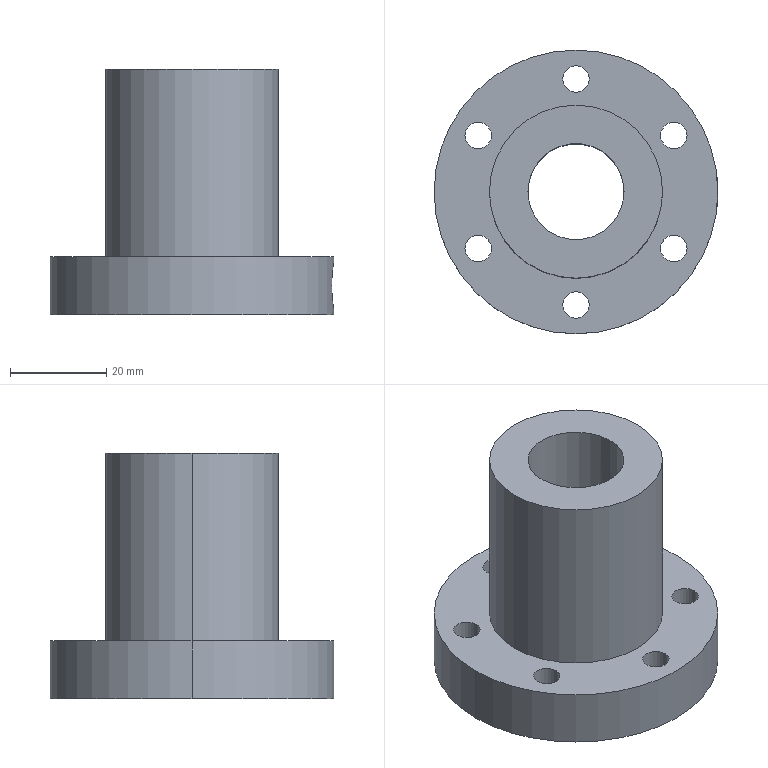Part | SolidWorks | features BaseBody 1 | 1 solid | 44 faces | box 59 x 59 x 51 mm | volume 51895 mm3 | cylinder 34 | plane 10 | commonest cylinder face diameters 5.5 x12 9.5 x12 8 x2 10 x2 20 x2 36 x2
STEP:
#1=CARTESIAN_POINT('',(-18.,0.,51.));
#2=VERTEX_POINT('',#1);
#3=CARTESIAN_POINT('',(18.,0.,51.));
#4=VERTEX_POINT('',#3);
#5=CARTESIAN_POINT('',(0.,0.,51.));
#6=DIRECTION('',(0.,0.,-1.));
#7=DIRECTION('',(-1.,0.,0.));
#8=AXIS2_PLACEMENT_3D('',#5,#6,#7);
#9=CIRCLE('',#8,18.);
#10=EDGE_CURVE('',#2,#4,#9,.T.);
#11=ORIENTED_EDGE('',*,*,#10,.T.);
#12=CARTESIAN_POINT('',(18.,0.,12.));
#13=VERTEX_POINT('',#12);
#14=CARTESIAN_POINT('',(18.,0.,-13.427));
#15=DIRECTION('',(0.,0.,-1.));
#16=VECTOR('',#15,1000.);
#17=LINE('',#14,#16);
#18=EDGE_CURVE('',#4,#13,#17,.T.);
#19=ORIENTED_EDGE('',*,*,#18,.T.);
#20=CARTESIAN_POINT('',(-18.,0.,12.));
#21=VERTEX_POINT('',#20);
#22=CARTESIAN_POINT('',(0.,0.,12.));
#23=DIRECTION('',(0.,0.,1.));
#24=DIRECTION('',(-1.,0.,0.));
#25=AXIS2_PLACEMENT_3D('',#22,#23,#24);
#26=CIRCLE('',#25,18.);
#27=EDGE_CURVE('',#13,#21,#26,.T.);
#28=ORIENTED_EDGE('',*,*,#27,.T.);
#29=CARTESIAN_POINT('',(-18.,0.,-13.427));
#30=DIRECTION('',(0.,0.,-1.));
#31=VECTOR('',#30,1000.);
#32=LINE('',#29,#31);
#33=EDGE_CURVE('',#2,#21,#32,.T.);
#34=ORIENTED_EDGE('',*,*,#33,.F.);
#35=EDGE_LOOP('',(#11,#19,#28,#34));
#36=FACE_OUTER_BOUND('',#35,.T.);
#37=CARTESIAN_POINT('',(0.,0.,-13.427));
#38=DIRECTION('',(0.,0.,-1.));
#39=DIRECTION('',(-1.,0.,0.));
#40=AXIS2_PLACEMENT_3D('',#37,#38,#39);
#41=CYLINDRICAL_SURFACE('',#40,18.);
#42=ADVANCED_FACE('',(#36),#41,.T.);
#43=CARTESIAN_POINT('',(-10.,0.,51.));
#44=VERTEX_POINT('',#43);
#45=CARTESIAN_POINT('',(10.,0.,51.));
#46=VERTEX_POINT('',#45);
#47=CARTESIAN_POINT('',(0.,0.,51.));
#48=DIRECTION('',(0.,0.,1.));
#49=DIRECTION('',(-1.,0.,0.));
#50=AXIS2_PLACEMENT_3D('',#47,#48,#49);
#51=CIRCLE('',#50,10.);
#52=EDGE_CURVE('',#44,#46,#51,.T.);
#53=ORIENTED_EDGE('',*,*,#52,.T.);
#54=CARTESIAN_POINT('',(10.,0.,10.));
#55=VERTEX_POINT('',#54);
#56=CARTESIAN_POINT('',(10.,0.,-13.427));
#57=DIRECTION('',(0.,0.,-1.));
#58=VECTOR('',#57,1000.);
#59=LINE('',#56,#58);
#60=EDGE_CURVE('',#46,#55,#59,.T.);
#61=ORIENTED_EDGE('',*,*,#60,.T.);
#62=CARTESIAN_POINT('',(10.,0.,2.));
#63=VERTEX_POINT('',#62);
#64=CARTESIAN_POINT('',(10.,0.,2.));
#65=CARTESIAN_POINT('',(10.,-0.2672,2.));
#66=CARTESIAN_POINT('',(9.989,-0.5294,2.026));
#67=CARTESIAN_POINT('',(9.949,-1.044,2.13));
#68=CARTESIAN_POINT('',(9.918,-1.3,2.208));
#69=CARTESIAN_POINT('',(9.843,-1.783,2.41));
#70=CARTESIAN_POINT('',(9.798,-2.012,2.533));
#71=CARTESIAN_POINT('',(9.699,-2.445,2.823));
#72=CARTESIAN_POINT('',(9.645,-2.647,2.99));
#73=CARTESIAN_POINT('',(9.538,-3.012,3.355));
#74=CARTESIAN_POINT('',(9.483,-3.177,3.555));
#75=CARTESIAN_POINT('',(9.381,-3.468,3.989));
#76=CARTESIAN_POINT('',(9.334,-3.59,4.218));
#77=CARTESIAN_POINT('',(9.254,-3.791,4.698));
#78=CARTESIAN_POINT('',(9.221,-3.869,4.952));
#79=CARTESIAN_POINT('',(9.177,-3.973,5.469));
#80=CARTESIAN_POINT('',(9.165,-4.,5.731));
#81=CARTESIAN_POINT('',(9.165,-4.,6.259));
#82=CARTESIAN_POINT('',(9.177,-3.974,6.527));
#83=CARTESIAN_POINT('',(9.221,-3.871,7.042));
#84=CARTESIAN_POINT('',(9.253,-3.794,7.293));
#85=CARTESIAN_POINT('',(9.333,-3.592,7.781));
#86=CARTESIAN_POINT('',(9.381,-3.468,8.009));
#87=CARTESIAN_POINT('',(9.482,-3.18,8.44));
#88=CARTESIAN_POINT('',(9.537,-3.013,8.643));
#89=CARTESIAN_POINT('',(9.645,-2.647,9.01));
#90=CARTESIAN_POINT('',(9.698,-2.448,9.174));
#91=CARTESIAN_POINT('',(9.797,-2.017,9.464));
#92=CARTESIAN_POINT('',(9.843,-1.784,9.59));
#93=CARTESIAN_POINT('',(9.918,-1.303,9.791));
#94=CARTESIAN_POINT('',(9.948,-1.054,9.868));
#95=CARTESIAN_POINT('',(9.989,-0.5328,9.973));
#96=CARTESIAN_POINT('',(10.,-0.2673,10.));
#97=CARTESIAN_POINT('',(10.,0.,10.));
#98=B_SPLINE_CURVE_WITH_KNOTS('',3,(#64,#65,#66,#67,#68,#69,#70,#71,#72,#73,#74,#75,#76,#77,#78,#79,#80,#81,#82,#83,#84,#85,#86,#87,#88,#89,#90,#91,#92,#93,#94,#95,#96,#97),.UNSPECIFIED.,.F.,.F.,(4,2,2,2,2,2,2,2,2,2,2,2,2,2,2,2,4),(0.,0.0007896,0.001579,0.002369,0.003158,0.003948,0.004738,0.005527,0.006317,0.007107,0.007896,0.008686,0.009475,0.01027,0.01105,0.01184,0.01263),.UNSPECIFIED.);
#99=EDGE_CURVE('',#63,#55,#98,.T.);
#100=ORIENTED_EDGE('',*,*,#99,.F.);
#101=CARTESIAN_POINT('',(10.,0.,0.));
#102=VERTEX_POINT('',#101);
#103=CARTESIAN_POINT('',(10.,0.,-13.427));
#104=DIRECTION('',(0.,0.,-1.));
#105=VECTOR('',#104,1000.);
#106=LINE('',#103,#105);
#107=EDGE_CURVE('',#63,#102,#106,.T.);
#108=ORIENTED_EDGE('',*,*,#107,.T.);
#109=CARTESIAN_POINT('',(-10.,0.,0.));
#110=VERTEX_POINT('',#109);
#111=CARTESIAN_POINT('',(0.,0.,0.));
#112=DIRECTION('',(0.,0.,1.));
#113=DIRECTION('',(-1.,0.,0.));
#114=AXIS2_PLACEMENT_3D('',#111,#112,#113);
#115=CIRCLE('',#114,10.);
#116=EDGE_CURVE('',#110,#102,#115,.T.);
#117=ORIENTED_EDGE('',*,*,#116,.F.);
#118=CARTESIAN_POINT('',(-10.,0.,-13.427));
#119=DIRECTION('',(0.,0.,-1.));
#120=VECTOR('',#119,1000.);
#121=LINE('',#118,#120);
#122=EDGE_CURVE('',#44,#110,#121,.T.);
#123=ORIENTED_EDGE('',*,*,#122,.F.);
#124=EDGE_LOOP('',(#53,#61,#100,#108,#117,#123));
#125=FACE_OUTER_BOUND('',#124,.T.);
#126=CARTESIAN_POINT('',(0.,0.,-13.427));
#127=DIRECTION('',(0.,0.,-1.));
#128=DIRECTION('',(-1.,0.,0.));
#129=AXIS2_PLACEMENT_3D('',#126,#127,#128);
#130=CYLINDRICAL_SURFACE('',#129,10.);
#131=ADVANCED_FACE('',(#125),#130,.F.);
#132=CARTESIAN_POINT('',(-29.5,0.,12.));
#133=VERTEX_POINT('',#132);
#134=CARTESIAN_POINT('',(29.5,0.,12.));
#135=VERTEX_POINT('',#134);
#136=CARTESIAN_POINT('',(0.,0.,12.));
#137=DIRECTION('',(0.,0.,-1.));
#138=DIRECTION('',(-1.,0.,0.));
#139=AXIS2_PLACEMENT_3D('',#136,#137,#138);
#140=CIRCLE('',#139,29.5);
#141=EDGE_CURVE('',#133,#135,#140,.T.);
#142=ORIENTED_EDGE('',*,*,#141,.T.);
#143=CARTESIAN_POINT('',(29.5,0.,11.));
#144=VERTEX_POINT('',#143);
#145=CARTESIAN_POINT('',(29.5,0.,-13.427));
#146=DIRECTION('',(0.,0.,-1.));
#147=VECTOR('',#146,1000.);
#148=LINE('',#145,#147);
#149=EDGE_CURVE('',#135,#144,#148,.T.);
#150=ORIENTED_EDGE('',*,*,#149,.T.);
#151=CARTESIAN_POINT('',(29.5,0.,1.));
#152=VERTEX_POINT('',#151);
#153=CARTESIAN_POINT('',(29.5,0.,11.));
#154=CARTESIAN_POINT('',(29.5,0.3309,11.));
#155=CARTESIAN_POINT('',(29.494,0.6562,10.967));
#156=CARTESIAN_POINT('',(29.479,1.136,10.872));
#157=CARTESIAN_POINT('',(29.472,1.295,10.832));
#158=CARTESIAN_POINT('',(29.457,1.609,10.737));
#159=CARTESIAN_POINT('',(29.448,1.765,10.681));
#160=CARTESIAN_POINT('',(29.418,2.219,10.493));
#161=CARTESIAN_POINT('',(29.395,2.506,10.339));
#162=CARTESIAN_POINT('',(29.343,3.049,9.976));
#163=CARTESIAN_POINT('',(29.315,3.306,9.766));
#164=CARTESIAN_POINT('',(29.26,3.766,9.305));
#165=CARTESIAN_POINT('',(29.232,3.973,9.054));
#166=CARTESIAN_POINT('',(29.18,4.338,8.508));
#167=CARTESIAN_POINT('',(29.156,4.493,8.218));
#168=CARTESIAN_POINT('',(29.117,4.743,7.617));
#169=CARTESIAN_POINT('',(29.1,4.839,7.301));
#170=CARTESIAN_POINT('',(29.079,4.968,6.655));
#171=CARTESIAN_POINT('',(29.073,5.,6.331));
#172=CARTESIAN_POINT('',(29.073,5.,5.677));
#173=CARTESIAN_POINT('',(29.079,4.968,5.345));
#174=CARTESIAN_POINT('',(29.1,4.84,4.704));
#175=CARTESIAN_POINT('',(29.116,4.746,4.392));
#176=CARTESIAN_POINT('',(29.146,4.558,3.937));
#177=CARTESIAN_POINT('',(29.157,4.487,3.787));
#178=CARTESIAN_POINT('',(29.18,4.332,3.498));
#179=CARTESIAN_POINT('',(29.193,4.248,3.358));
#180=CARTESIAN_POINT('',(29.231,3.977,2.953));
#181=CARTESIAN_POINT('',(29.259,3.77,2.699));
#182=CARTESIAN_POINT('',(29.315,3.305,2.234));
#183=CARTESIAN_POINT('',(29.343,3.053,2.027));
#184=CARTESIAN_POINT('',(29.394,2.513,1.665));
#185=CARTESIAN_POINT('',(29.418,2.22,1.508));
#186=CARTESIAN_POINT('',(29.457,1.616,1.257));
#187=CARTESIAN_POINT('',(29.473,1.304,1.162));
#188=CARTESIAN_POINT('',(29.494,0.6622,1.033));
#189=CARTESIAN_POINT('',(29.5,0.3309,1.));
#190=CARTESIAN_POINT('',(29.5,0.,1.));
#191=B_SPLINE_CURVE_WITH_KNOTS('',3,(#153,#154,#155,#156,#157,#158,#159,#160,#161,#162,#163,#164,#165,#166,#167,#168,#169,#170,#171,#172,#173,#174,#175,#176,#177,#178,#179,#180,#181,#182,#183,#184,#185,#186,#187,#188,#189,#190),.UNSPECIFIED.,.F.,.F.,(4,2,2,2,2,2,2,2,2,2,2,2,2,2,2,2,2,2,4),(0.,0.0009785,0.001468,0.001957,0.002936,0.003914,0.004893,0.005871,0.00685,0.007828,0.008807,0.009785,0.01027,0.01076,0.01174,0.01272,0.0137,0.01468,0.01566),.UNSPECIFIED.);
#192=EDGE_CURVE('',#144,#152,#191,.T.);
#193=ORIENTED_EDGE('',*,*,#192,.T.);
#194=CARTESIAN_POINT('',(29.5,0.,0.));
#195=VERTEX_POINT('',#194);
#196=CARTESIAN_POINT('',(29.5,0.,-13.427));
#197=DIRECTION('',(0.,0.,-1.));
#198=VECTOR('',#197,1000.);
#199=LINE('',#196,#198);
#200=EDGE_CURVE('',#152,#195,#199,.T.);
#201=ORIENTED_EDGE('',*,*,#200,.T.);
#202=CARTESIAN_POINT('',(-29.5,0.,0.));
#203=VERTEX_POINT('',#202);
#204=CARTESIAN_POINT('',(0.,0.,0.));
#205=DIRECTION('',(0.,0.,1.));
#206=DIRECTION('',(-1.,0.,0.));
#207=AXIS2_PLACEMENT_3D('',#204,#205,#206);
#208=CIRCLE('',#207,29.5);
#209=EDGE_CURVE('',#195,#203,#208,.T.);
#210=ORIENTED_EDGE('',*,*,#209,.T.);
#211=CARTESIAN_POINT('',(-29.5,0.,-13.427));
#212=DIRECTION('',(0.,0.,-1.));
#213=VECTOR('',#212,1000.);
#214=LINE('',#211,#213);
#215=EDGE_CURVE('',#133,#203,#214,.T.);
#216=ORIENTED_EDGE('',*,*,#215,.F.);
#217=EDGE_LOOP('',(#142,#150,#193,#201,#210,#216));
#218=FACE_OUTER_BOUND('',#217,.T.);
#219=CARTESIAN_POINT('',(0.,0.,-13.427));
#220=DIRECTION('',(0.,0.,-1.));
#221=DIRECTION('',(-1.,0.,0.));
#222=AXIS2_PLACEMENT_3D('',#219,#220,#221);
#223=CYLINDRICAL_SURFACE('',#222,29.5);
#224=ADVANCED_FACE('',(#218),#223,.T.);
#225=CARTESIAN_POINT('',(-2.75,23.5,5.5));
#226=VERTEX_POINT('',#225);
#227=CARTESIAN_POINT('',(2.75,23.5,5.5));
#228=VERTEX_POINT('',#227);
#229=CARTESIAN_POINT('',(0.,23.5,5.5));
#230=DIRECTION('',(0.,0.,1.));
#231=DIRECTION('',(1.,0.,0.));
#232=AXIS2_PLACEMENT_3D('',#229,#230,#231);
#233=CIRCLE('',#232,2.75);
#234=EDGE_CURVE('',#226,#228,#233,.T.);
#235=ORIENTED_EDGE('',*,*,#234,.F.);
#236=CARTESIAN_POINT('',(-2.75,23.5,12.));
#237=VERTEX_POINT('',#236);
#238=CARTESIAN_POINT('',(-2.75,23.5,17.));
#239=DIRECTION('',(0.,0.,1.));
#240=VECTOR('',#239,1000.);
#241=LINE('',#238,#240);
#242=EDGE_CURVE('',#226,#237,#241,.T.);
#243=ORIENTED_EDGE('',*,*,#242,.T.);
#244=CARTESIAN_POINT('',(2.75,23.5,12.));
#245=VERTEX_POINT('',#244);
#246=CARTESIAN_POINT('',(0.,23.5,12.));
#247=DIRECTION('',(0.,0.,1.));
#248=DIRECTION('',(1.,0.,0.));
#249=AXIS2_PLACEMENT_3D('',#246,#247,#248);
#250=CIRCLE('',#249,2.75);
#251=EDGE_CURVE('',#237,#245,#250,.T.);
#252=ORIENTED_EDGE('',*,*,#251,.T.);
#253=CARTESIAN_POINT('',(2.75,23.5,17.));
#254=DIRECTION('',(0.,0.,1.));
#255=VECTOR('',#254,1000.);
#256=LINE('',#253,#255);
#257=EDGE_CURVE('',#228,#245,#256,.T.);
#258=ORIENTED_EDGE('',*,*,#257,.F.);
#259=EDGE_LOOP('',(#235,#243,#252,#258));
#260=FACE_OUTER_BOUND('',#259,.T.);
#261=CARTESIAN_POINT('',(0.,23.5,17.));
#262=DIRECTION('',(0.,0.,1.));
#263=DIRECTION('',(1.,0.,0.));
#264=AXIS2_PLACEMENT_3D('',#261,#262,#263);
#265=CYLINDRICAL_SURFACE('',#264,2.75);
#266=ADVANCED_FACE('',(#260),#265,.F.);
#267=CARTESIAN_POINT('',(-23.102,11.75,5.5));
#268=VERTEX_POINT('',#267);
#269=CARTESIAN_POINT('',(-17.602,11.75,5.5));
#270=VERTEX_POINT('',#269);
#271=CARTESIAN_POINT('',(-20.352,11.75,5.5));
#272=DIRECTION('',(0.,0.,1.));
#273=DIRECTION('',(1.,0.,0.));
#274=AXIS2_PLACEMENT_3D('',#271,#272,#273);
#275=CIRCLE('',#274,2.75);
#276=EDGE_CURVE('',#268,#270,#275,.T.);
#277=ORIENTED_EDGE('',*,*,#276,.F.);
#278=CARTESIAN_POINT('',(-23.102,11.75,12.));
#279=VERTEX_POINT('',#278);
#280=CARTESIAN_POINT('',(-23.102,11.75,17.));
#281=DIRECTION('',(0.,0.,1.));
#282=VECTOR('',#281,1000.);
#283=LINE('',#280,#282);
#284=EDGE_CURVE('',#268,#279,#283,.T.);
#285=ORIENTED_EDGE('',*,*,#284,.T.);
#286=CARTESIAN_POINT('',(-17.602,11.75,12.));
#287=VERTEX_POINT('',#286);
#288=CARTESIAN_POINT('',(-20.352,11.75,12.));
#289=DIRECTION('',(0.,0.,1.));
#290=DIRECTION('',(1.,0.,0.));
#291=AXIS2_PLACEMENT_3D('',#288,#289,#290);
#292=CIRCLE('',#291,2.75);
#293=EDGE_CURVE('',#279,#287,#292,.T.);
#294=ORIENTED_EDGE('',*,*,#293,.T.);
#295=CARTESIAN_POINT('',(-17.602,11.75,17.));
#296=DIRECTION('',(0.,0.,1.));
#297=VECTOR('',#296,1000.);
#298=LINE('',#295,#297);
#299=EDGE_CURVE('',#270,#287,#298,.T.);
#300=ORIENTED_EDGE('',*,*,#299,.F.);
#301=EDGE_LOOP('',(#277,#285,#294,#300));
#302=FACE_OUTER_BOUND('',#301,.T.);
#303=CARTESIAN_POINT('',(-20.352,11.75,17.));
#304=DIRECTION('',(0.,0.,1.));
#305=DIRECTION('',(1.,0.,0.));
#306=AXIS2_PLACEMENT_3D('',#303,#304,#305);
#307=CYLINDRICAL_SURFACE('',#306,2.75);
#308=ADVANCED_FACE('',(#302),#307,.F.);
#309=CARTESIAN_POINT('',(-23.102,-11.75,5.5));
#310=VERTEX_POINT('',#309);
#311=CARTESIAN_POINT('',(-17.602,-11.75,5.5));
#312=VERTEX_POINT('',#311);
#313=CARTESIAN_POINT('',(-20.352,-11.75,5.5));
#314=DIRECTION('',(0.,0.,1.));
#315=DIRECTION('',(1.,0.,0.));
#316=AXIS2_PLACEMENT_3D('',#313,#314,#315);
#317=CIRCLE('',#316,2.75);
#318=EDGE_CURVE('',#310,#312,#317,.T.);
#319=ORIENTED_EDGE('',*,*,#318,.F.);
#320=CARTESIAN_POINT('',(-23.102,-11.75,12.));
#321=VERTEX_POINT('',#320);
#322=CARTESIAN_POINT('',(-23.102,-11.75,17.));
#323=DIRECTION('',(0.,0.,1.));
#324=VECTOR('',#323,1000.);
#325=LINE('',#322,#324);
#326=EDGE_CURVE('',#310,#321,#325,.T.);
#327=ORIENTED_EDGE('',*,*,#326,.T.);
#328=CARTESIAN_POINT('',(-17.602,-11.75,12.));
#329=VERTEX_POINT('',#328);
#330=CARTESIAN_POINT('',(-20.352,-11.75,12.));
#331=DIRECTION('',(0.,0.,1.));
#332=DIRECTION('',(1.,0.,0.));
#333=AXIS2_PLACEMENT_3D('',#330,#331,#332);
#334=CIRCLE('',#333,2.75);
#335=EDGE_CURVE('',#321,#329,#334,.T.);
#336=ORIENTED_EDGE('',*,*,#335,.T.);
#337=CARTESIAN_POINT('',(-17.602,-11.75,17.));
#338=DIRECTION('',(0.,0.,1.));
#339=VECTOR('',#338,1000.);
#340=LINE('',#337,#339);
#341=EDGE_CURVE('',#312,#329,#340,.T.);
#342=ORIENTED_EDGE('',*,*,#341,.F.);
#343=EDGE_LOOP('',(#319,#327,#336,#342));
#344=FACE_OUTER_BOUND('',#343,.T.);
#345=CARTESIAN_POINT('',(-20.352,-11.75,17.));
#346=DIRECTION('',(0.,0.,1.));
#347=DIRECTION('',(1.,0.,0.));
#348=AXIS2_PLACEMENT_3D('',#345,#346,#347);
#349=CYLINDRICAL_SURFACE('',#348,2.75);
#350=ADVANCED_FACE('',(#344),#349,.F.);
#351=CARTESIAN_POINT('',(-2.75,-23.5,5.5));
#352=VERTEX_POINT('',#351);
#353=CARTESIAN_POINT('',(2.75,-23.5,5.5));
#354=VERTEX_POINT('',#353);
#355=CARTESIAN_POINT('',(0.,-23.5,5.5));
#356=DIRECTION('',(0.,0.,1.));
#357=DIRECTION('',(1.,0.,0.));
#358=AXIS2_PLACEMENT_3D('',#355,#356,#357);
#359=CIRCLE('',#358,2.75);
#360=EDGE_CURVE('',#352,#354,#359,.T.);
#361=ORIENTED_EDGE('',*,*,#360,.F.);
#362=CARTESIAN_POINT('',(-2.75,-23.5,12.));
#363=VERTEX_POINT('',#362);
#364=CARTESIAN_POINT('',(-2.75,-23.5,17.));
#365=DIRECTION('',(0.,0.,1.));
#366=VECTOR('',#365,1000.);
#367=LINE('',#364,#366);
#368=EDGE_CURVE('',#352,#363,#367,.T.);
#369=ORIENTED_EDGE('',*,*,#368,.T.);
#370=CARTESIAN_POINT('',(2.75,-23.5,12.));
#371=VERTEX_POINT('',#370);
#372=CARTESIAN_POINT('',(0.,-23.5,12.));
#373=DIRECTION('',(0.,0.,1.));
#374=DIRECTION('',(1.,0.,0.));
#375=AXIS2_PLACEMENT_3D('',#372,#373,#374);
#376=CIRCLE('',#375,2.75);
#377=EDGE_CURVE('',#363,#371,#376,.T.);
#378=ORIENTED_EDGE('',*,*,#377,.T.);
#379=CARTESIAN_POINT('',(2.75,-23.5,17.));
#380=DIRECTION('',(0.,0.,1.));
#381=VECTOR('',#380,1000.);
#382=LINE('',#379,#381);
#383=EDGE_CURVE('',#354,#371,#382,.T.);
#384=ORIENTED_EDGE('',*,*,#383,.F.);
#385=EDGE_LOOP('',(#361,#369,#378,#384));
#386=FACE_OUTER_BOUND('',#385,.T.);
#387=CARTESIAN_POINT('',(0.,-23.5,17.));
#388=DIRECTION('',(0.,0.,1.));
#389=DIRECTION('',(1.,0.,0.));
#390=AXIS2_PLACEMENT_3D('',#387,#388,#389);
#391=CYLINDRICAL_SURFACE('',#390,2.75);
#392=ADVANCED_FACE('',(#386),#391,.F.);
#393=CARTESIAN_POINT('',(17.602,-11.75,5.5));
#394=VERTEX_POINT('',#393);
#395=CARTESIAN_POINT('',(23.102,-11.75,5.5));
#396=VERTEX_POINT('',#395);
#397=CARTESIAN_POINT('',(20.352,-11.75,5.5));
#398=DIRECTION('',(0.,0.,1.));
#399=DIRECTION('',(1.,0.,0.));
#400=AXIS2_PLACEMENT_3D('',#397,#398,#399);
#401=CIRCLE('',#400,2.75);
#402=EDGE_CURVE('',#394,#396,#401,.T.);
#403=ORIENTED_EDGE('',*,*,#402,.F.);
#404=CARTESIAN_POINT('',(17.602,-11.75,12.));
#405=VERTEX_POINT('',#404);
#406=CARTESIAN_POINT('',(17.602,-11.75,17.));
#407=DIRECTION('',(0.,0.,1.));
#408=VECTOR('',#407,1000.);
#409=LINE('',#406,#408);
#410=EDGE_CURVE('',#394,#405,#409,.T.);
#411=ORIENTED_EDGE('',*,*,#410,.T.);
#412=CARTESIAN_POINT('',(23.102,-11.75,12.));
#413=VERTEX_POINT('',#412);
#414=CARTESIAN_POINT('',(20.352,-11.75,12.));
#415=DIRECTION('',(0.,0.,1.));
#416=DIRECTION('',(1.,0.,0.));
#417=AXIS2_PLACEMENT_3D('',#414,#415,#416);
#418=CIRCLE('',#417,2.75);
#419=EDGE_CURVE('',#405,#413,#418,.T.);
#420=ORIENTED_EDGE('',*,*,#419,.T.);
#421=CARTESIAN_POINT('',(23.102,-11.75,17.));
#422=DIRECTION('',(0.,0.,1.));
#423=VECTOR('',#422,1000.);
#424=LINE('',#421,#423);
#425=EDGE_CURVE('',#396,#413,#424,.T.);
#426=ORIENTED_EDGE('',*,*,#425,.F.);
#427=EDGE_LOOP('',(#403,#411,#420,#426));
#428=FACE_OUTER_BOUND('',#427,.T.);
#429=CARTESIAN_POINT('',(20.352,-11.75,17.));
#430=DIRECTION('',(0.,0.,1.));
#431=DIRECTION('',(1.,0.,0.));
#432=AXIS2_PLACEMENT_3D('',#429,#430,#431);
#433=CYLINDRICAL_SURFACE('',#432,2.75);
#434=ADVANCED_FACE('',(#428),#433,.F.);
#435=CARTESIAN_POINT('',(17.602,11.75,5.5));
#436=VERTEX_POINT('',#435);
#437=CARTESIAN_POINT('',(23.102,11.75,5.5));
#438=VERTEX_POINT('',#437);
#439=CARTESIAN_POINT('',(20.352,11.75,5.5));
#440=DIRECTION('',(0.,0.,1.));
#441=DIRECTION('',(1.,0.,0.));
#442=AXIS2_PLACEMENT_3D('',#439,#440,#441);
#443=CIRCLE('',#442,2.75);
#444=EDGE_CURVE('',#436,#438,#443,.T.);
#445=ORIENTED_EDGE('',*,*,#444,.F.);
#446=CARTESIAN_POINT('',(17.602,11.75,12.));
#447=VERTEX_POINT('',#446);
#448=CARTESIAN_POINT('',(17.602,11.75,17.));
#449=DIRECTION('',(0.,0.,1.));
#450=VECTOR('',#449,1000.);
#451=LINE('',#448,#450);
#452=EDGE_CURVE('',#436,#447,#451,.T.);
#453=ORIENTED_EDGE('',*,*,#452,.T.);
#454=CARTESIAN_POINT('',(23.102,11.75,12.));
#455=VERTEX_POINT('',#454);
#456=CARTESIAN_POINT('',(20.352,11.75,12.));
#457=DIRECTION('',(0.,0.,1.));
#458=DIRECTION('',(1.,0.,0.));
#459=AXIS2_PLACEMENT_3D('',#456,#457,#458);
#460=CIRCLE('',#459,2.75);
#461=EDGE_CURVE('',#447,#455,#460,.T.);
#462=ORIENTED_EDGE('',*,*,#461,.T.);
#463=CARTESIAN_POINT('',(23.102,11.75,17.));
#464=DIRECTION('',(0.,0.,1.));
#465=VECTOR('',#464,1000.);
#466=LINE('',#463,#465);
#467=EDGE_CURVE('',#438,#455,#466,.T.);
#468=ORIENTED_EDGE('',*,*,#467,.F.);
#469=EDGE_LOOP('',(#445,#453,#462,#468));
#470=FACE_OUTER_BOUND('',#469,.T.);
#471=CARTESIAN_POINT('',(20.352,11.75,17.));
#472=DIRECTION('',(0.,0.,1.));
#473=DIRECTION('',(1.,0.,0.));
#474=AXIS2_PLACEMENT_3D('',#471,#472,#473);
#475=CYLINDRICAL_SURFACE('',#474,2.75);
#476=ADVANCED_FACE('',(#470),#475,.F.);
#477=CARTESIAN_POINT('',(4.75,23.5,0.));
#478=VERTEX_POINT('',#477);
#479=CARTESIAN_POINT('',(-4.75,23.5,0.));
#480=VERTEX_POINT('',#479);
#481=CARTESIAN_POINT('',(0.,23.5,0.));
#482=DIRECTION('',(0.,0.,-1.));
#483=DIRECTION('',(1.,0.,0.));
#484=AXIS2_PLACEMENT_3D('',#481,#482,#483);
#485=CIRCLE('',#484,4.75);
#486=EDGE_CURVE('',#478,#480,#485,.T.);
#487=ORIENTED_EDGE('',*,*,#486,.T.);
#488=CARTESIAN_POINT('',(-4.75,23.5,5.5));
#489=VERTEX_POINT('',#488);
#490=CARTESIAN_POINT('',(-4.75,23.5,0.));
#491=DIRECTION('',(0.,0.,1.));
#492=VECTOR('',#491,1000.);
#493=LINE('',#490,#492);
#494=EDGE_CURVE('',#480,#489,#493,.T.);
#495=ORIENTED_EDGE('',*,*,#494,.T.);
#496=CARTESIAN_POINT('',(4.75,23.5,5.5));
#497=VERTEX_POINT('',#496);
#498=CARTESIAN_POINT('',(0.,23.5,5.5));
#499=DIRECTION('',(0.,0.,1.));
#500=DIRECTION('',(1.,0.,0.));
#501=AXIS2_PLACEMENT_3D('',#498,#499,#500);
#502=CIRCLE('',#501,4.75);
#503=EDGE_CURVE('',#489,#497,#502,.T.);
#504=ORIENTED_EDGE('',*,*,#503,.T.);
#505=CARTESIAN_POINT('',(4.75,23.5,0.));
#506=DIRECTION('',(0.,0.,1.));
#507=VECTOR('',#506,1000.);
#508=LINE('',#505,#507);
#509=EDGE_CURVE('',#478,#497,#508,.T.);
#510=ORIENTED_EDGE('',*,*,#509,.F.);
#511=EDGE_LOOP('',(#487,#495,#504,#510));
#512=FACE_OUTER_BOUND('',#511,.T.);
#513=CARTESIAN_POINT('',(0.,23.5,0.));
#514=DIRECTION('',(0.,0.,1.));
#515=DIRECTION('',(1.,0.,0.));
#516=AXIS2_PLACEMENT_3D('',#513,#514,#515);
#517=CYLINDRICAL_SURFACE('',#516,4.75);
#518=ADVANCED_FACE('',(#512),#517,.F.);
#519=CARTESIAN_POINT('',(-15.602,11.75,0.));
#520=VERTEX_POINT('',#519);
#521=CARTESIAN_POINT('',(-25.102,11.75,0.));
#522=VERTEX_POINT('',#521);
#523=CARTESIAN_POINT('',(-20.352,11.75,0.));
#524=DIRECTION('',(0.,0.,-1.));
#525=DIRECTION('',(1.,0.,0.));
#526=AXIS2_PLACEMENT_3D('',#523,#524,#525);
#527=CIRCLE('',#526,4.75);
#528=EDGE_CURVE('',#520,#522,#527,.T.);
#529=ORIENTED_EDGE('',*,*,#528,.T.);
#530=CARTESIAN_POINT('',(-25.102,11.75,5.5));
#531=VERTEX_POINT('',#530);
#532=CARTESIAN_POINT('',(-25.102,11.75,0.));
#533=DIRECTION('',(0.,0.,1.));
#534=VECTOR('',#533,1000.);
#535=LINE('',#532,#534);
#536=EDGE_CURVE('',#522,#531,#535,.T.);
#537=ORIENTED_EDGE('',*,*,#536,.T.);
#538=CARTESIAN_POINT('',(-15.602,11.75,5.5));
#539=VERTEX_POINT('',#538);
#540=CARTESIAN_POINT('',(-20.352,11.75,5.5));
#541=DIRECTION('',(0.,0.,1.));
#542=DIRECTION('',(1.,0.,0.));
#543=AXIS2_PLACEMENT_3D('',#540,#541,#542);
#544=CIRCLE('',#543,4.75);
#545=EDGE_CURVE('',#531,#539,#544,.T.);
#546=ORIENTED_EDGE('',*,*,#545,.T.);
#547=CARTESIAN_POINT('',(-15.602,11.75,0.));
#548=DIRECTION('',(0.,0.,1.));
#549=VECTOR('',#548,1000.);
#550=LINE('',#547,#549);
#551=EDGE_CURVE('',#520,#539,#550,.T.);
#552=ORIENTED_EDGE('',*,*,#551,.F.);
#553=EDGE_LOOP('',(#529,#537,#546,#552));
#554=FACE_OUTER_BOUND('',#553,.T.);
#555=CARTESIAN_POINT('',(-20.352,11.75,0.));
#556=DIRECTION('',(0.,0.,1.));
#557=DIRECTION('',(1.,0.,0.));
#558=AXIS2_PLACEMENT_3D('',#555,#556,#557);
#559=CYLINDRICAL_SURFACE('',#558,4.75);
#560=ADVANCED_FACE('',(#554),#559,.F.);
#561=CARTESIAN_POINT('',(-15.602,-11.75,0.));
#562=VERTEX_POINT('',#561);
#563=CARTESIAN_POINT('',(-25.102,-11.75,0.));
#564=VERTEX_POINT('',#563);
#565=CARTESIAN_POINT('',(-20.352,-11.75,0.));
#566=DIRECTION('',(0.,0.,-1.));
#567=DIRECTION('',(1.,0.,0.));
#568=AXIS2_PLACEMENT_3D('',#565,#566,#567);
#569=CIRCLE('',#568,4.75);
#570=EDGE_CURVE('',#562,#564,#569,.T.);
#571=ORIENTED_EDGE('',*,*,#570,.T.);
#572=CARTESIAN_POINT('',(-25.102,-11.75,5.5));
#573=VERTEX_POINT('',#572);
#574=CARTESIAN_POINT('',(-25.102,-11.75,0.));
#575=DIRECTION('',(0.,0.,1.));
#576=VECTOR('',#575,1000.);
#577=LINE('',#574,#576);
#578=EDGE_CURVE('',#564,#573,#577,.T.);
#579=ORIENTED_EDGE('',*,*,#578,.T.);
#580=CARTESIAN_POINT('',(-15.602,-11.75,5.5));
#581=VERTEX_POINT('',#580);
#582=CARTESIAN_POINT('',(-20.352,-11.75,5.5));
#583=DIRECTION('',(0.,0.,1.));
#584=DIRECTION('',(1.,0.,0.));
#585=AXIS2_PLACEMENT_3D('',#582,#583,#584);
#586=CIRCLE('',#585,4.75);
#587=EDGE_CURVE('',#573,#581,#586,.T.);
#588=ORIENTED_EDGE('',*,*,#587,.T.);
#589=CARTESIAN_POINT('',(-15.602,-11.75,0.));
#590=DIRECTION('',(0.,0.,1.));
#591=VECTOR('',#590,1000.);
#592=LINE('',#589,#591);
#593=EDGE_CURVE('',#562,#581,#592,.T.);
#594=ORIENTED_EDGE('',*,*,#593,.F.);
#595=EDGE_LOOP('',(#571,#579,#588,#594));
#596=FACE_OUTER_BOUND('',#595,.T.);
#597=CARTESIAN_POINT('',(-20.352,-11.75,0.));
#598=DIRECTION('',(0.,0.,1.));
#599=DIRECTION('',(1.,0.,0.));
#600=AXIS2_PLACEMENT_3D('',#597,#598,#599);
#601=CYLINDRICAL_SURFACE('',#600,4.75);
#602=ADVANCED_FACE('',(#596),#601,.F.);
#603=CARTESIAN_POINT('',(4.75,-23.5,0.));
#604=VERTEX_POINT('',#603);
#605=CARTESIAN_POINT('',(-4.75,-23.5,0.));
#606=VERTEX_POINT('',#605);
#607=CARTESIAN_POINT('',(0.,-23.5,0.));
#608=DIRECTION('',(0.,0.,-1.));
#609=DIRECTION('',(1.,0.,0.));
#610=AXIS2_PLACEMENT_3D('',#607,#608,#609);
#611=CIRCLE('',#610,4.75);
#612=EDGE_CURVE('',#604,#606,#611,.T.);
#613=ORIENTED_EDGE('',*,*,#612,.T.);
#614=CARTESIAN_POINT('',(-4.75,-23.5,5.5));
#615=VERTEX_POINT('',#614);
#616=CARTESIAN_POINT('',(-4.75,-23.5,0.));
#617=DIRECTION('',(0.,0.,1.));
#618=VECTOR('',#617,1000.);
#619=LINE('',#616,#618);
#620=EDGE_CURVE('',#606,#615,#619,.T.);
#621=ORIENTED_EDGE('',*,*,#620,.T.);
#622=CARTESIAN_POINT('',(4.75,-23.5,5.5));
#623=VERTEX_POINT('',#622);
#624=CARTESIAN_POINT('',(0.,-23.5,5.5));
#625=DIRECTION('',(0.,0.,1.));
#626=DIRECTION('',(1.,0.,0.));
#627=AXIS2_PLACEMENT_3D('',#624,#625,#626);
#628=CIRCLE('',#627,4.75);
#629=EDGE_CURVE('',#615,#623,#628,.T.);
#630=ORIENTED_EDGE('',*,*,#629,.T.);
#631=CARTESIAN_POINT('',(4.75,-23.5,0.));
#632=DIRECTION('',(0.,0.,1.));
#633=VECTOR('',#632,1000.);
#634=LINE('',#631,#633);
#635=EDGE_CURVE('',#604,#623,#634,.T.);
#636=ORIENTED_EDGE('',*,*,#635,.F.);
#637=EDGE_LOOP('',(#613,#621,#630,#636));
#638=FACE_OUTER_BOUND('',#637,.T.);
#639=CARTESIAN_POINT('',(0.,-23.5,0.));
#640=DIRECTION('',(0.,0.,1.));
#641=DIRECTION('',(1.,0.,0.));
#642=AXIS2_PLACEMENT_3D('',#639,#640,#641);
#643=CYLINDRICAL_SURFACE('',#642,4.75);
#644=ADVANCED_FACE('',(#638),#643,.F.);
#645=CARTESIAN_POINT('',(25.102,-11.75,0.));
#646=VERTEX_POINT('',#645);
#647=CARTESIAN_POINT('',(15.602,-11.75,0.));
#648=VERTEX_POINT('',#647);
#649=CARTESIAN_POINT('',(20.352,-11.75,0.));
#650=DIRECTION('',(0.,0.,-1.));
#651=DIRECTION('',(1.,0.,0.));
#652=AXIS2_PLACEMENT_3D('',#649,#650,#651);
#653=CIRCLE('',#652,4.75);
#654=EDGE_CURVE('',#646,#648,#653,.T.);
#655=ORIENTED_EDGE('',*,*,#654,.T.);
#656=CARTESIAN_POINT('',(15.602,-11.75,5.5));
#657=VERTEX_POINT('',#656);
#658=CARTESIAN_POINT('',(15.602,-11.75,0.));
#659=DIRECTION('',(0.,0.,1.));
#660=VECTOR('',#659,1000.);
#661=LINE('',#658,#660);
#662=EDGE_CURVE('',#648,#657,#661,.T.);
#663=ORIENTED_EDGE('',*,*,#662,.T.);
#664=CARTESIAN_POINT('',(25.102,-11.75,5.5));
#665=VERTEX_POINT('',#664);
#666=CARTESIAN_POINT('',(20.352,-11.75,5.5));
#667=DIRECTION('',(0.,0.,1.));
#668=DIRECTION('',(1.,0.,0.));
#669=AXIS2_PLACEMENT_3D('',#666,#667,#668);
#670=CIRCLE('',#669,4.75);
#671=EDGE_CURVE('',#657,#665,#670,.T.);
#672=ORIENTED_EDGE('',*,*,#671,.T.);
#673=CARTESIAN_POINT('',(25.102,-11.75,0.));
#674=DIRECTION('',(0.,0.,1.));
#675=VECTOR('',#674,1000.);
#676=LINE('',#673,#675);
#677=EDGE_CURVE('',#646,#665,#676,.T.);
#678=ORIENTED_EDGE('',*,*,#677,.F.);
#679=EDGE_LOOP('',(#655,#663,#672,#678));
#680=FACE_OUTER_BOUND('',#679,.T.);
#681=CARTESIAN_POINT('',(20.352,-11.75,0.));
#682=DIRECTION('',(0.,0.,1.));
#683=DIRECTION('',(1.,0.,0.));
#684=AXIS2_PLACEMENT_3D('',#681,#682,#683);
#685=CYLINDRICAL_SURFACE('',#684,4.75);
#686=ADVANCED_FACE('',(#680),#685,.F.);
#687=CARTESIAN_POINT('',(25.102,11.75,0.));
#688=VERTEX_POINT('',#687);
#689=CARTESIAN_POINT('',(15.602,11.75,0.));
#690=VERTEX_POINT('',#689);
#691=CARTESIAN_POINT('',(20.352,11.75,0.));
#692=DIRECTION('',(0.,0.,-1.));
#693=DIRECTION('',(1.,0.,0.));
#694=AXIS2_PLACEMENT_3D('',#691,#692,#693);
#695=CIRCLE('',#694,4.75);
#696=EDGE_CURVE('',#688,#690,#695,.T.);
#697=ORIENTED_EDGE('',*,*,#696,.T.);
#698=CARTESIAN_POINT('',(15.602,11.75,5.5));
#699=VERTEX_POINT('',#698);
#700=CARTESIAN_POINT('',(15.602,11.75,0.));
#701=DIRECTION('',(0.,0.,1.));
#702=VECTOR('',#701,1000.);
#703=LINE('',#700,#702);
#704=EDGE_CURVE('',#690,#699,#703,.T.);
#705=ORIENTED_EDGE('',*,*,#704,.T.);
#706=CARTESIAN_POINT('',(25.102,11.75,5.5));
#707=VERTEX_POINT('',#706);
#708=CARTESIAN_POINT('',(20.352,11.75,5.5));
#709=DIRECTION('',(0.,0.,1.));
#710=DIRECTION('',(1.,0.,0.));
#711=AXIS2_PLACEMENT_3D('',#708,#709,#710);
#712=CIRCLE('',#711,4.75);
#713=EDGE_CURVE('',#699,#707,#712,.T.);
#714=ORIENTED_EDGE('',*,*,#713,.T.);
#715=CARTESIAN_POINT('',(25.102,11.75,0.));
#716=DIRECTION('',(0.,0.,1.));
#717=VECTOR('',#716,1000.);
#718=LINE('',#715,#717);
#719=EDGE_CURVE('',#688,#707,#718,.T.);
#720=ORIENTED_EDGE('',*,*,#719,.F.);
#721=EDGE_LOOP('',(#697,#705,#714,#720));
#722=FACE_OUTER_BOUND('',#721,.T.);
#723=CARTESIAN_POINT('',(20.352,11.75,0.));
#724=DIRECTION('',(0.,0.,1.));
#725=DIRECTION('',(1.,0.,0.));
#726=AXIS2_PLACEMENT_3D('',#723,#724,#725);
#727=CYLINDRICAL_SURFACE('',#726,4.75);
#728=ADVANCED_FACE('',(#722),#727,.F.);
#729=CARTESIAN_POINT('',(17.5,0.,11.));
#730=VERTEX_POINT('',#729);
#731=CARTESIAN_POINT('',(17.5,0.,1.));
#732=VERTEX_POINT('',#731);
#733=CARTESIAN_POINT('',(17.5,0.,6.));
#734=DIRECTION('',(1.,0.,0.));
#735=DIRECTION('',(0.,0.,-1.));
#736=AXIS2_PLACEMENT_3D('',#733,#734,#735);
#737=CIRCLE('',#736,5.);
#738=EDGE_CURVE('',#730,#732,#737,.T.);
#739=ORIENTED_EDGE('',*,*,#738,.F.);
#740=CARTESIAN_POINT('',(17.5,0.,11.));
#741=DIRECTION('',(1.,0.,0.));
#742=VECTOR('',#741,1000.);
#743=LINE('',#740,#742);
#744=EDGE_CURVE('',#730,#144,#743,.T.);
#745=ORIENTED_EDGE('',*,*,#744,.T.);
#746=CARTESIAN_POINT('',(29.5,0.,1.));
#747=CARTESIAN_POINT('',(29.5,-0.3309,1.));
#748=CARTESIAN_POINT('',(29.494,-0.6562,1.033));
#749=CARTESIAN_POINT('',(29.479,-1.136,1.128));
#750=CARTESIAN_POINT('',(29.472,-1.295,1.168));
#751=CARTESIAN_POINT('',(29.457,-1.609,1.263));
#752=CARTESIAN_POINT('',(29.448,-1.765,1.319));
#753=CARTESIAN_POINT('',(29.418,-2.219,1.507));
#754=CARTESIAN_POINT('',(29.395,-2.506,1.661));
#755=CARTESIAN_POINT('',(29.343,-3.049,2.024));
#756=CARTESIAN_POINT('',(29.315,-3.306,2.234));
#757=CARTESIAN_POINT('',(29.26,-3.766,2.695));
#758=CARTESIAN_POINT('',(29.232,-3.973,2.946));
#759=CARTESIAN_POINT('',(29.18,-4.338,3.492));
#760=CARTESIAN_POINT('',(29.156,-4.493,3.782));
#761=CARTESIAN_POINT('',(29.117,-4.743,4.383));
#762=CARTESIAN_POINT('',(29.1,-4.839,4.699));
#763=CARTESIAN_POINT('',(29.079,-4.968,5.345));
#764=CARTESIAN_POINT('',(29.073,-5.,5.669));
#765=CARTESIAN_POINT('',(29.073,-5.,6.323));
#766=CARTESIAN_POINT('',(29.079,-4.968,6.655));
#767=CARTESIAN_POINT('',(29.1,-4.84,7.296));
#768=CARTESIAN_POINT('',(29.116,-4.746,7.608));
#769=CARTESIAN_POINT('',(29.146,-4.558,8.063));
#770=CARTESIAN_POINT('',(29.157,-4.487,8.213));
#771=CARTESIAN_POINT('',(29.18,-4.332,8.502));
#772=CARTESIAN_POINT('',(29.193,-4.248,8.642));
#773=CARTESIAN_POINT('',(29.231,-3.977,9.047));
#774=CARTESIAN_POINT('',(29.259,-3.77,9.301));
#775=CARTESIAN_POINT('',(29.315,-3.305,9.766));
#776=CARTESIAN_POINT('',(29.343,-3.053,9.973));
#777=CARTESIAN_POINT('',(29.394,-2.513,10.335));
#778=CARTESIAN_POINT('',(29.418,-2.22,10.492));
#779=CARTESIAN_POINT('',(29.457,-1.616,10.743));
#780=CARTESIAN_POINT('',(29.473,-1.304,10.838));
#781=CARTESIAN_POINT('',(29.494,-0.6622,10.967));
#782=CARTESIAN_POINT('',(29.5,-0.3309,11.));
#783=CARTESIAN_POINT('',(29.5,0.,11.));
#784=B_SPLINE_CURVE_WITH_KNOTS('',3,(#746,#747,#748,#749,#750,#751,#752,#753,#754,#755,#756,#757,#758,#759,#760,#761,#762,#763,#764,#765,#766,#767,#768,#769,#770,#771,#772,#773,#774,#775,#776,#777,#778,#779,#780,#781,#782,#783),.UNSPECIFIED.,.F.,.F.,(4,2,2,2,2,2,2,2,2,2,2,2,2,2,2,2,2,2,4),(0.01566,0.01664,0.01712,0.01761,0.01859,0.01957,0.02055,0.02153,0.02251,0.02348,0.02446,0.02544,0.02593,0.02642,0.0274,0.02838,0.02936,0.03033,0.03131),.UNSPECIFIED.);
#785=EDGE_CURVE('',#152,#144,#784,.T.);
#786=ORIENTED_EDGE('',*,*,#785,.F.);
#787=CARTESIAN_POINT('',(17.5,0.,1.));
#788=DIRECTION('',(1.,0.,0.));
#789=VECTOR('',#788,1000.);
#790=LINE('',#787,#789);
#791=EDGE_CURVE('',#732,#152,#790,.T.);
#792=ORIENTED_EDGE('',*,*,#791,.F.);
#793=EDGE_LOOP('',(#739,#745,#786,#792));
#794=FACE_OUTER_BOUND('',#793,.T.);
#795=CARTESIAN_POINT('',(17.5,0.,6.));
#796=DIRECTION('',(1.,0.,0.));
#797=DIRECTION('',(0.,0.,-1.));
#798=AXIS2_PLACEMENT_3D('',#795,#796,#797);
#799=CYLINDRICAL_SURFACE('',#798,5.);
#800=ADVANCED_FACE('',(#794),#799,.F.);
#801=CARTESIAN_POINT('',(17.5,0.,10.));
#802=VERTEX_POINT('',#801);
#803=CARTESIAN_POINT('',(17.5,0.,2.));
#804=VERTEX_POINT('',#803);
#805=CARTESIAN_POINT('',(17.5,0.,6.));
#806=DIRECTION('',(1.,0.,0.));
#807=DIRECTION('',(0.,0.,1.));
#808=AXIS2_PLACEMENT_3D('',#805,#806,#807);
#809=CIRCLE('',#808,4.);
#810=EDGE_CURVE('',#802,#804,#809,.T.);
#811=ORIENTED_EDGE('',*,*,#810,.T.);
#812=CARTESIAN_POINT('',(17.5,0.,2.));
#813=DIRECTION('',(-1.,0.,0.));
#814=VECTOR('',#813,1000.);
#815=LINE('',#812,#814);
#816=EDGE_CURVE('',#804,#63,#815,.T.);
#817=ORIENTED_EDGE('',*,*,#816,.T.);
#818=ORIENTED_EDGE('',*,*,#99,.T.);
#819=CARTESIAN_POINT('',(17.5,0.,10.));
#820=DIRECTION('',(-1.,0.,0.));
#821=VECTOR('',#820,1000.);
#822=LINE('',#819,#821);
#823=EDGE_CURVE('',#802,#55,#822,.T.);
#824=ORIENTED_EDGE('',*,*,#823,.F.);
#825=EDGE_LOOP('',(#811,#817,#818,#824));
#826=FACE_OUTER_BOUND('',#825,.T.);
#827=CARTESIAN_POINT('',(17.5,0.,6.));
#828=DIRECTION('',(-1.,0.,0.));
#829=DIRECTION('',(0.,0.,1.));
#830=AXIS2_PLACEMENT_3D('',#827,#828,#829);
#831=CYLINDRICAL_SURFACE('',#830,4.);
#832=ADVANCED_FACE('',(#826),#831,.F.);
#833=ORIENTED_EDGE('',*,*,#810,.F.);
#834=CARTESIAN_POINT('',(17.5,0.,6.));
#835=DIRECTION('',(1.,0.,0.));
#836=DIRECTION('',(0.,0.,1.));
#837=AXIS2_PLACEMENT_3D('',#834,#835,#836);
#838=CIRCLE('',#837,4.);
#839=EDGE_CURVE('',#804,#802,#838,.T.);
#840=ORIENTED_EDGE('',*,*,#839,.F.);
#841=EDGE_LOOP('',(#833,#840));
#842=FACE_BOUND('',#841,.T.);
#843=CARTESIAN_POINT('',(17.5,0.,6.));
#844=DIRECTION('',(1.,0.,0.));
#845=DIRECTION('',(0.,0.,-1.));
#846=AXIS2_PLACEMENT_3D('',#843,#844,#845);
#847=CIRCLE('',#846,5.);
#848=EDGE_CURVE('',#732,#730,#847,.T.);
#849=ORIENTED_EDGE('',*,*,#848,.T.);
#850=ORIENTED_EDGE('',*,*,#738,.T.);
#851=EDGE_LOOP('',(#849,#850));
#852=FACE_OUTER_BOUND('',#851,.T.);
#853=CARTESIAN_POINT('',(17.5,0.,6.));
#854=DIRECTION('',(-1.,0.,0.));
#855=DIRECTION('',(0.,0.,1.));
#856=AXIS2_PLACEMENT_3D('',#853,#854,#855);
#857=PLANE('',#856);
#858=ADVANCED_FACE('',(#842,#852),#857,.F.);
#859=CARTESIAN_POINT('',(20.352,11.75,5.5));
#860=DIRECTION('',(0.,0.,1.));
#861=DIRECTION('',(1.,0.,0.));
#862=AXIS2_PLACEMENT_3D('',#859,#860,#861);
#863=CIRCLE('',#862,2.75);
#864=EDGE_CURVE('',#438,#436,#863,.T.);
#865=ORIENTED_EDGE('',*,*,#864,.T.);
#866=ORIENTED_EDGE('',*,*,#444,.T.);
#867=EDGE_LOOP('',(#865,#866));
#868=FACE_BOUND('',#867,.T.);
#869=CARTESIAN_POINT('',(20.352,11.75,5.5));
#870=DIRECTION('',(0.,0.,1.));
#871=DIRECTION('',(1.,0.,0.));
#872=AXIS2_PLACEMENT_3D('',#869,#870,#871);
#873=CIRCLE('',#872,4.75);
#874=EDGE_CURVE('',#707,#699,#873,.T.);
#875=ORIENTED_EDGE('',*,*,#874,.F.);
#876=ORIENTED_EDGE('',*,*,#713,.F.);
#877=EDGE_LOOP('',(#875,#876));
#878=FACE_OUTER_BOUND('',#877,.T.);
#879=CARTESIAN_POINT('',(20.352,11.75,5.5));
#880=DIRECTION('',(0.,0.,1.));
#881=DIRECTION('',(1.,0.,0.));
#882=AXIS2_PLACEMENT_3D('',#879,#880,#881);
#883=PLANE('',#882);
#884=ADVANCED_FACE('',(#868,#878),#883,.F.);
#885=CARTESIAN_POINT('',(20.352,-11.75,5.5));
#886=DIRECTION('',(0.,0.,1.));
#887=DIRECTION('',(1.,0.,0.));
#888=AXIS2_PLACEMENT_3D('',#885,#886,#887);
#889=CIRCLE('',#888,2.75);
#890=EDGE_CURVE('',#396,#394,#889,.T.);
#891=ORIENTED_EDGE('',*,*,#890,.T.);
#892=ORIENTED_EDGE('',*,*,#402,.T.);
#893=EDGE_LOOP('',(#891,#892));
#894=FACE_BOUND('',#893,.T.);
#895=CARTESIAN_POINT('',(20.352,-11.75,5.5));
#896=DIRECTION('',(0.,0.,1.));
#897=DIRECTION('',(1.,0.,0.));
#898=AXIS2_PLACEMENT_3D('',#895,#896,#897);
#899=CIRCLE('',#898,4.75);
#900=EDGE_CURVE('',#665,#657,#899,.T.);
#901=ORIENTED_EDGE('',*,*,#900,.F.);
#902=ORIENTED_EDGE('',*,*,#671,.F.);
#903=EDGE_LOOP('',(#901,#902));
#904=FACE_OUTER_BOUND('',#903,.T.);
#905=CARTESIAN_POINT('',(20.352,-11.75,5.5));
#906=DIRECTION('',(0.,0.,1.));
#907=DIRECTION('',(1.,0.,0.));
#908=AXIS2_PLACEMENT_3D('',#905,#906,#907);
#909=PLANE('',#908);
#910=ADVANCED_FACE('',(#894,#904),#909,.F.);
#911=CARTESIAN_POINT('',(0.,-23.5,5.5));
#912=DIRECTION('',(0.,0.,1.));
#913=DIRECTION('',(1.,0.,0.));
#914=AXIS2_PLACEMENT_3D('',#911,#912,#913);
#915=CIRCLE('',#914,2.75);
#916=EDGE_CURVE('',#354,#352,#915,.T.);
#917=ORIENTED_EDGE('',*,*,#916,.T.);
#918=ORIENTED_EDGE('',*,*,#360,.T.);
#919=EDGE_LOOP('',(#917,#918));
#920=FACE_BOUND('',#919,.T.);
#921=CARTESIAN_POINT('',(0.,-23.5,5.5));
#922=DIRECTION('',(0.,0.,1.));
#923=DIRECTION('',(1.,0.,0.));
#924=AXIS2_PLACEMENT_3D('',#921,#922,#923);
#925=CIRCLE('',#924,4.75);
#926=EDGE_CURVE('',#623,#615,#925,.T.);
#927=ORIENTED_EDGE('',*,*,#926,.F.);
#928=ORIENTED_EDGE('',*,*,#629,.F.);
#929=EDGE_LOOP('',(#927,#928));
#930=FACE_OUTER_BOUND('',#929,.T.);
#931=CARTESIAN_POINT('',(0.,-23.5,5.5));
#932=DIRECTION('',(0.,0.,1.));
#933=DIRECTION('',(1.,0.,0.));
#934=AXIS2_PLACEMENT_3D('',#931,#932,#933);
#935=PLANE('',#934);
#936=ADVANCED_FACE('',(#920,#930),#935,.F.);
#937=CARTESIAN_POINT('',(-20.352,-11.75,5.5));
#938=DIRECTION('',(0.,0.,1.));
#939=DIRECTION('',(1.,0.,0.));
#940=AXIS2_PLACEMENT_3D('',#937,#938,#939);
#941=CIRCLE('',#940,2.75);
#942=EDGE_CURVE('',#312,#310,#941,.T.);
#943=ORIENTED_EDGE('',*,*,#942,.T.);
#944=ORIENTED_EDGE('',*,*,#318,.T.);
#945=EDGE_LOOP('',(#943,#944));
#946=FACE_BOUND('',#945,.T.);
#947=CARTESIAN_POINT('',(-20.352,-11.75,5.5));
#948=DIRECTION('',(0.,0.,1.));
#949=DIRECTION('',(1.,0.,0.));
#950=AXIS2_PLACEMENT_3D('',#947,#948,#949);
#951=CIRCLE('',#950,4.75);
#952=EDGE_CURVE('',#581,#573,#951,.T.);
#953=ORIENTED_EDGE('',*,*,#952,.F.);
#954=ORIENTED_EDGE('',*,*,#587,.F.);
#955=EDGE_LOOP('',(#953,#954));
#956=FACE_OUTER_BOUND('',#955,.T.);
#957=CARTESIAN_POINT('',(-20.352,-11.75,5.5));
#958=DIRECTION('',(0.,0.,1.));
#959=DIRECTION('',(1.,0.,0.));
#960=AXIS2_PLACEMENT_3D('',#957,#958,#959);
#961=PLANE('',#960);
#962=ADVANCED_FACE('',(#946,#956),#961,.F.);
#963=CARTESIAN_POINT('',(-20.352,11.75,5.5));
#964=DIRECTION('',(0.,0.,1.));
#965=DIRECTION('',(1.,0.,0.));
#966=AXIS2_PLACEMENT_3D('',#963,#964,#965);
#967=CIRCLE('',#966,2.75);
#968=EDGE_CURVE('',#270,#268,#967,.T.);
#969=ORIENTED_EDGE('',*,*,#968,.T.);
#970=ORIENTED_EDGE('',*,*,#276,.T.);
#971=EDGE_LOOP('',(#969,#970));
#972=FACE_BOUND('',#971,.T.);
#973=CARTESIAN_POINT('',(-20.352,11.75,5.5));
#974=DIRECTION('',(0.,0.,1.));
#975=DIRECTION('',(1.,0.,0.));
#976=AXIS2_PLACEMENT_3D('',#973,#974,#975);
#977=CIRCLE('',#976,4.75);
#978=EDGE_CURVE('',#539,#531,#977,.T.);
#979=ORIENTED_EDGE('',*,*,#978,.F.);
#980=ORIENTED_EDGE('',*,*,#545,.F.);
#981=EDGE_LOOP('',(#979,#980));
#982=FACE_OUTER_BOUND('',#981,.T.);
#983=CARTESIAN_POINT('',(-20.352,11.75,5.5));
#984=DIRECTION('',(0.,0.,1.));
#985=DIRECTION('',(1.,0.,0.));
#986=AXIS2_PLACEMENT_3D('',#983,#984,#985);
#987=PLANE('',#986);
#988=ADVANCED_FACE('',(#972,#982),#987,.F.);
#989=CARTESIAN_POINT('',(0.,23.5,5.5));
#990=DIRECTION('',(0.,0.,1.));
#991=DIRECTION('',(1.,0.,0.));
#992=AXIS2_PLACEMENT_3D('',#989,#990,#991);
#993=CIRCLE('',#992,2.75);
#994=EDGE_CURVE('',#228,#226,#993,.T.);
#995=ORIENTED_EDGE('',*,*,#994,.T.);
#996=ORIENTED_EDGE('',*,*,#234,.T.);
#997=EDGE_LOOP('',(#995,#996));
#998=FACE_BOUND('',#997,.T.);
#999=CARTESIAN_POINT('',(0.,23.5,5.5));
#1000=DIRECTION('',(0.,0.,1.));
#1001=DIRECTION('',(1.,0.,0.));
#1002=AXIS2_PLACEMENT_3D('',#999,#1000,#1001);
#1003=CIRCLE('',#1002,4.75);
#1004=EDGE_CURVE('',#497,#489,#1003,.T.);
#1005=ORIENTED_EDGE('',*,*,#1004,.F.);
#1006=ORIENTED_EDGE('',*,*,#503,.F.);
#1007=EDGE_LOOP('',(#1005,#1006));
#1008=FACE_OUTER_BOUND('',#1007,.T.);
#1009=CARTESIAN_POINT('',(0.,23.5,5.5));
#1010=DIRECTION('',(0.,0.,1.));
#1011=DIRECTION('',(1.,0.,0.));
#1012=AXIS2_PLACEMENT_3D('',#1009,#1010,#1011);
#1013=PLANE('',#1012);
#1014=ADVANCED_FACE('',(#998,#1008),#1013,.F.);
#1015=ORIENTED_EDGE('',*,*,#696,.F.);
#1016=CARTESIAN_POINT('',(20.352,11.75,0.));
#1017=DIRECTION('',(0.,0.,-1.));
#1018=DIRECTION('',(1.,0.,0.));
#1019=AXIS2_PLACEMENT_3D('',#1016,#1017,#1018);
#1020=CIRCLE('',#1019,4.75);
#1021=EDGE_CURVE('',#690,#688,#1020,.T.);
#1022=ORIENTED_EDGE('',*,*,#1021,.F.);
#1023=EDGE_LOOP('',(#1015,#1022));
#1024=FACE_BOUND('',#1023,.T.);
#1025=ORIENTED_EDGE('',*,*,#654,.F.);
#1026=CARTESIAN_POINT('',(20.352,-11.75,0.));
#1027=DIRECTION('',(0.,0.,-1.));
#1028=DIRECTION('',(1.,0.,0.));
#1029=AXIS2_PLACEMENT_3D('',#1026,#1027,#1028);
#1030=CIRCLE('',#1029,4.75);
#1031=EDGE_CURVE('',#648,#646,#1030,.T.);
#1032=ORIENTED_EDGE('',*,*,#1031,.F.);
#1033=EDGE_LOOP('',(#1025,#1032));
#1034=FACE_BOUND('',#1033,.T.);
#1035=ORIENTED_EDGE('',*,*,#612,.F.);
#1036=CARTESIAN_POINT('',(0.,-23.5,0.));
#1037=DIRECTION('',(0.,0.,-1.));
#1038=DIRECTION('',(1.,0.,0.));
#1039=AXIS2_PLACEMENT_3D('',#1036,#1037,#1038);
#1040=CIRCLE('',#1039,4.75);
#1041=EDGE_CURVE('',#606,#604,#1040,.T.);
#1042=ORIENTED_EDGE('',*,*,#1041,.F.);
#1043=EDGE_LOOP('',(#1035,#1042));
#1044=FACE_BOUND('',#1043,.T.);
#1045=ORIENTED_EDGE('',*,*,#570,.F.);
#1046=CARTESIAN_POINT('',(-20.352,-11.75,0.));
#1047=DIRECTION('',(0.,0.,-1.));
#1048=DIRECTION('',(1.,0.,0.));
#1049=AXIS2_PLACEMENT_3D('',#1046,#1047,#1048);
#1050=CIRCLE('',#1049,4.75);
#1051=EDGE_CURVE('',#564,#562,#1050,.T.);
#1052=ORIENTED_EDGE('',*,*,#1051,.F.);
#1053=EDGE_LOOP('',(#1045,#1052));
#1054=FACE_BOUND('',#1053,.T.);
#1055=ORIENTED_EDGE('',*,*,#528,.F.);
#1056=CARTESIAN_POINT('',(-20.352,11.75,0.));
#1057=DIRECTION('',(0.,0.,-1.));
#1058=DIRECTION('',(1.,0.,0.));
#1059=AXIS2_PLACEMENT_3D('',#1056,#1057,#1058);
#1060=CIRCLE('',#1059,4.75);
#1061=EDGE_CURVE('',#522,#520,#1060,.T.);
#1062=ORIENTED_EDGE('',*,*,#1061,.F.);
#1063=EDGE_LOOP('',(#1055,#1062));
#1064=FACE_BOUND('',#1063,.T.);
#1065=ORIENTED_EDGE('',*,*,#486,.F.);
#1066=CARTESIAN_POINT('',(0.,23.5,0.));
#1067=DIRECTION('',(0.,0.,-1.));
#1068=DIRECTION('',(1.,0.,0.));
#1069=AXIS2_PLACEMENT_3D('',#1066,#1067,#1068);
#1070=CIRCLE('',#1069,4.75);
#1071=EDGE_CURVE('',#480,#478,#1070,.T.);
#1072=ORIENTED_EDGE('',*,*,#1071,.F.);
#1073=EDGE_LOOP('',(#1065,#1072));
#1074=FACE_BOUND('',#1073,.T.);
#1075=ORIENTED_EDGE('',*,*,#116,.T.);
#1076=CARTESIAN_POINT('',(0.,0.,0.));
#1077=DIRECTION('',(0.,0.,1.));
#1078=DIRECTION('',(-1.,0.,0.));
#1079=AXIS2_PLACEMENT_3D('',#1076,#1077,#1078);
#1080=CIRCLE('',#1079,10.);
#1081=EDGE_CURVE('',#102,#110,#1080,.T.);
#1082=ORIENTED_EDGE('',*,*,#1081,.T.);
#1083=EDGE_LOOP('',(#1075,#1082));
#1084=FACE_BOUND('',#1083,.T.);
#1085=CARTESIAN_POINT('',(0.,0.,0.));
#1086=DIRECTION('',(0.,0.,1.));
#1087=DIRECTION('',(-1.,0.,0.));
#1088=AXIS2_PLACEMENT_3D('',#1085,#1086,#1087);
#1089=CIRCLE('',#1088,29.5);
#1090=EDGE_CURVE('',#203,#195,#1089,.T.);
#1091=ORIENTED_EDGE('',*,*,#1090,.F.);
#1092=ORIENTED_EDGE('',*,*,#209,.F.);
#1093=EDGE_LOOP('',(#1091,#1092));
#1094=FACE_OUTER_BOUND('',#1093,.T.);
#1095=CARTESIAN_POINT('',(0.,29.5,0.));
#1096=DIRECTION('',(0.,0.,1.));
#1097=DIRECTION('',(1.,0.,0.));
#1098=AXIS2_PLACEMENT_3D('',#1095,#1096,#1097);
#1099=PLANE('',#1098);
#1100=ADVANCED_FACE('',(#1024,#1034,#1044,#1054,#1064,#1074,#1084,#1094),#1099,.F.);
#1101=CARTESIAN_POINT('',(20.352,11.75,12.));
#1102=DIRECTION('',(0.,0.,1.));
#1103=DIRECTION('',(1.,0.,0.));
#1104=AXIS2_PLACEMENT_3D('',#1101,#1102,#1103);
#1105=CIRCLE('',#1104,2.75);
#1106=EDGE_CURVE('',#455,#447,#1105,.T.);
#1107=ORIENTED_EDGE('',*,*,#1106,.F.);
#1108=ORIENTED_EDGE('',*,*,#461,.F.);
#1109=EDGE_LOOP('',(#1107,#1108));
#1110=FACE_BOUND('',#1109,.T.);
#1111=CARTESIAN_POINT('',(20.352,-11.75,12.));
#1112=DIRECTION('',(0.,0.,1.));
#1113=DIRECTION('',(1.,0.,0.));
#1114=AXIS2_PLACEMENT_3D('',#1111,#1112,#1113);
#1115=CIRCLE('',#1114,2.75);
#1116=EDGE_CURVE('',#413,#405,#1115,.T.);
#1117=ORIENTED_EDGE('',*,*,#1116,.F.);
#1118=ORIENTED_EDGE('',*,*,#419,.F.);
#1119=EDGE_LOOP('',(#1117,#1118));
#1120=FACE_BOUND('',#1119,.T.);
#1121=CARTESIAN_POINT('',(0.,-23.5,12.));
#1122=DIRECTION('',(0.,0.,1.));
#1123=DIRECTION('',(1.,0.,0.));
#1124=AXIS2_PLACEMENT_3D('',#1121,#1122,#1123);
#1125=CIRCLE('',#1124,2.75);
#1126=EDGE_CURVE('',#371,#363,#1125,.T.);
#1127=ORIENTED_EDGE('',*,*,#1126,.F.);
#1128=ORIENTED_EDGE('',*,*,#377,.F.);
#1129=EDGE_LOOP('',(#1127,#1128));
#1130=FACE_BOUND('',#1129,.T.);
#1131=CARTESIAN_POINT('',(-20.352,-11.75,12.));
#1132=DIRECTION('',(0.,0.,1.));
#1133=DIRECTION('',(1.,0.,0.));
#1134=AXIS2_PLACEMENT_3D('',#1131,#1132,#1133);
#1135=CIRCLE('',#1134,2.75);
#1136=EDGE_CURVE('',#329,#321,#1135,.T.);
#1137=ORIENTED_EDGE('',*,*,#1136,.F.);
#1138=ORIENTED_EDGE('',*,*,#335,.F.);
#1139=EDGE_LOOP('',(#1137,#1138));
#1140=FACE_BOUND('',#1139,.T.);
#1141=CARTESIAN_POINT('',(-20.352,11.75,12.));
#1142=DIRECTION('',(0.,0.,1.));
#1143=DIRECTION('',(1.,0.,0.));
#1144=AXIS2_PLACEMENT_3D('',#1141,#1142,#1143);
#1145=CIRCLE('',#1144,2.75);
#1146=EDGE_CURVE('',#287,#279,#1145,.T.);
#1147=ORIENTED_EDGE('',*,*,#1146,.F.);
#1148=ORIENTED_EDGE('',*,*,#293,.F.);
#1149=EDGE_LOOP('',(#1147,#1148));
#1150=FACE_BOUND('',#1149,.T.);
#1151=CARTESIAN_POINT('',(0.,23.5,12.));
#1152=DIRECTION('',(0.,0.,1.));
#1153=DIRECTION('',(1.,0.,0.));
#1154=AXIS2_PLACEMENT_3D('',#1151,#1152,#1153);
#1155=CIRCLE('',#1154,2.75);
#1156=EDGE_CURVE('',#245,#237,#1155,.T.);
#1157=ORIENTED_EDGE('',*,*,#1156,.F.);
#1158=ORIENTED_EDGE('',*,*,#251,.F.);
#1159=EDGE_LOOP('',(#1157,#1158));
#1160=FACE_BOUND('',#1159,.T.);
#1161=CARTESIAN_POINT('',(0.,0.,12.));
#1162=DIRECTION('',(0.,0.,1.));
#1163=DIRECTION('',(-1.,0.,0.));
#1164=AXIS2_PLACEMENT_3D('',#1161,#1162,#1163);
#1165=CIRCLE('',#1164,18.);
#1166=EDGE_CURVE('',#21,#13,#1165,.T.);
#1167=ORIENTED_EDGE('',*,*,#1166,.F.);
#1168=ORIENTED_EDGE('',*,*,#27,.F.);
#1169=EDGE_LOOP('',(#1167,#1168));
#1170=FACE_BOUND('',#1169,.T.);
#1171=ORIENTED_EDGE('',*,*,#141,.F.);
#1172=CARTESIAN_POINT('',(0.,0.,12.));
#1173=DIRECTION('',(0.,0.,-1.));
#1174=DIRECTION('',(-1.,0.,0.));
#1175=AXIS2_PLACEMENT_3D('',#1172,#1173,#1174);
#1176=CIRCLE('',#1175,29.5);
#1177=EDGE_CURVE('',#135,#133,#1176,.T.);
#1178=ORIENTED_EDGE('',*,*,#1177,.F.);
#1179=EDGE_LOOP('',(#1171,#1178));
#1180=FACE_OUTER_BOUND('',#1179,.T.);
#1181=CARTESIAN_POINT('',(0.,18.,12.));
#1182=DIRECTION('',(0.,0.,-1.));
#1183=DIRECTION('',(0.,-1.,0.));
#1184=AXIS2_PLACEMENT_3D('',#1181,#1182,#1183);
#1185=PLANE('',#1184);
#1186=ADVANCED_FACE('',(#1110,#1120,#1130,#1140,#1150,#1160,#1170,#1180),#1185,.F.);
#1187=ORIENTED_EDGE('',*,*,#52,.F.);
#1188=CARTESIAN_POINT('',(0.,0.,51.));
#1189=DIRECTION('',(0.,0.,1.));
#1190=DIRECTION('',(-1.,0.,0.));
#1191=AXIS2_PLACEMENT_3D('',#1188,#1189,#1190);
#1192=CIRCLE('',#1191,10.);
#1193=EDGE_CURVE('',#46,#44,#1192,.T.);
#1194=ORIENTED_EDGE('',*,*,#1193,.F.);
#1195=EDGE_LOOP('',(#1187,#1194));
#1196=FACE_BOUND('',#1195,.T.);
#1197=ORIENTED_EDGE('',*,*,#10,.F.);
#1198=CARTESIAN_POINT('',(0.,0.,51.));
#1199=DIRECTION('',(0.,0.,-1.));
#1200=DIRECTION('',(-1.,0.,0.));
#1201=AXIS2_PLACEMENT_3D('',#1198,#1199,#1200);
#1202=CIRCLE('',#1201,18.);
#1203=EDGE_CURVE('',#4,#2,#1202,.T.);
#1204=ORIENTED_EDGE('',*,*,#1203,.F.);
#1205=EDGE_LOOP('',(#1197,#1204));
#1206=FACE_OUTER_BOUND('',#1205,.T.);
#1207=CARTESIAN_POINT('',(0.,10.,51.));
#1208=DIRECTION('',(0.,0.,-1.));
#1209=DIRECTION('',(0.,-1.,0.));
#1210=AXIS2_PLACEMENT_3D('',#1207,#1208,#1209);
#1211=PLANE('',#1210);
#1212=ADVANCED_FACE('',(#1196,#1206),#1211,.F.);
#1213=ORIENTED_EDGE('',*,*,#816,.F.);
#1214=ORIENTED_EDGE('',*,*,#839,.T.);
#1215=ORIENTED_EDGE('',*,*,#823,.T.);
#1216=CARTESIAN_POINT('',(10.,0.,10.));
#1217=CARTESIAN_POINT('',(10.,0.2672,10.));
#1218=CARTESIAN_POINT('',(9.989,0.5294,9.974));
#1219=CARTESIAN_POINT('',(9.949,1.044,9.87));
#1220=CARTESIAN_POINT('',(9.918,1.3,9.792));
#1221=CARTESIAN_POINT('',(9.843,1.783,9.59));
#1222=CARTESIAN_POINT('',(9.798,2.012,9.467));
#1223=CARTESIAN_POINT('',(9.699,2.445,9.177));
#1224=CARTESIAN_POINT('',(9.645,2.647,9.01));
#1225=CARTESIAN_POINT('',(9.538,3.012,8.645));
#1226=CARTESIAN_POINT('',(9.483,3.177,8.445));
#1227=CARTESIAN_POINT('',(9.381,3.468,8.011));
#1228=CARTESIAN_POINT('',(9.334,3.59,7.782));
#1229=CARTESIAN_POINT('',(9.254,3.791,7.302));
#1230=CARTESIAN_POINT('',(9.221,3.869,7.048));
#1231=CARTESIAN_POINT('',(9.177,3.973,6.531));
#1232=CARTESIAN_POINT('',(9.165,4.,6.269));
#1233=CARTESIAN_POINT('',(9.165,4.,5.741));
#1234=CARTESIAN_POINT('',(9.177,3.974,5.473));
#1235=CARTESIAN_POINT('',(9.221,3.871,4.958));
#1236=CARTESIAN_POINT('',(9.253,3.794,4.707));
#1237=CARTESIAN_POINT('',(9.333,3.592,4.219));
#1238=CARTESIAN_POINT('',(9.381,3.468,3.991));
#1239=CARTESIAN_POINT('',(9.482,3.18,3.56));
#1240=CARTESIAN_POINT('',(9.537,3.013,3.357));
#1241=CARTESIAN_POINT('',(9.645,2.647,2.99));
#1242=CARTESIAN_POINT('',(9.698,2.448,2.826));
#1243=CARTESIAN_POINT('',(9.797,2.017,2.536));
#1244=CARTESIAN_POINT('',(9.843,1.784,2.41));
#1245=CARTESIAN_POINT('',(9.918,1.303,2.209));
#1246=CARTESIAN_POINT('',(9.948,1.054,2.132));
#1247=CARTESIAN_POINT('',(9.989,0.5328,2.027));
#1248=CARTESIAN_POINT('',(10.,0.2671,2.));
#1249=CARTESIAN_POINT('',(10.,0.,2.));
#1250=B_SPLINE_CURVE_WITH_KNOTS('',3,(#1216,#1217,#1218,#1219,#1220,#1221,#1222,#1223,#1224,#1225,#1226,#1227,#1228,#1229,#1230,#1231,#1232,#1233,#1234,#1235,#1236,#1237,#1238,#1239,#1240,#1241,#1242,#1243,#1244,#1245,#1246,#1247,#1248,#1249),.UNSPECIFIED.,.F.,.F.,(4,2,2,2,2,2,2,2,2,2,2,2,2,2,2,2,4),(0.01263,0.01342,0.01421,0.015,0.01579,0.01658,0.01737,0.01816,0.01895,0.01974,0.02053,0.02132,0.02211,0.0229,0.02369,0.02447,0.02526),.UNSPECIFIED.);
#1251=EDGE_CURVE('',#55,#63,#1250,.T.);
#1252=ORIENTED_EDGE('',*,*,#1251,.T.);
#1253=EDGE_LOOP('',(#1213,#1214,#1215,#1252));
#1254=FACE_OUTER_BOUND('',#1253,.T.);
#1255=CARTESIAN_POINT('',(17.5,0.,6.));
#1256=DIRECTION('',(-1.,0.,0.));
#1257=DIRECTION('',(0.,0.,1.));
#1258=AXIS2_PLACEMENT_3D('',#1255,#1256,#1257);
#1259=CYLINDRICAL_SURFACE('',#1258,4.);
#1260=ADVANCED_FACE('',(#1254),#1259,.F.);
#1261=ORIENTED_EDGE('',*,*,#744,.F.);
#1262=ORIENTED_EDGE('',*,*,#848,.F.);
#1263=ORIENTED_EDGE('',*,*,#791,.T.);
#1264=ORIENTED_EDGE('',*,*,#192,.F.);
#1265=EDGE_LOOP('',(#1261,#1262,#1263,#1264));
#1266=FACE_OUTER_BOUND('',#1265,.T.);
#1267=CARTESIAN_POINT('',(17.5,0.,6.));
#1268=DIRECTION('',(1.,0.,0.));
#1269=DIRECTION('',(0.,0.,-1.));
#1270=AXIS2_PLACEMENT_3D('',#1267,#1268,#1269);
#1271=CYLINDRICAL_SURFACE('',#1270,5.);
#1272=ADVANCED_FACE('',(#1266),#1271,.F.);
#1273=ORIENTED_EDGE('',*,*,#704,.F.);
#1274=ORIENTED_EDGE('',*,*,#1021,.T.);
#1275=ORIENTED_EDGE('',*,*,#719,.T.);
#1276=ORIENTED_EDGE('',*,*,#874,.T.);
#1277=EDGE_LOOP('',(#1273,#1274,#1275,#1276));
#1278=FACE_OUTER_BOUND('',#1277,.T.);
#1279=CARTESIAN_POINT('',(20.352,11.75,0.));
#1280=DIRECTION('',(0.,0.,1.));
#1281=DIRECTION('',(1.,0.,0.));
#1282=AXIS2_PLACEMENT_3D('',#1279,#1280,#1281);
#1283=CYLINDRICAL_SURFACE('',#1282,4.75);
#1284=ADVANCED_FACE('',(#1278),#1283,.F.);
#1285=ORIENTED_EDGE('',*,*,#662,.F.);
#1286=ORIENTED_EDGE('',*,*,#1031,.T.);
#1287=ORIENTED_EDGE('',*,*,#677,.T.);
#1288=ORIENTED_EDGE('',*,*,#900,.T.);
#1289=EDGE_LOOP('',(#1285,#1286,#1287,#1288));
#1290=FACE_OUTER_BOUND('',#1289,.T.);
#1291=CARTESIAN_POINT('',(20.352,-11.75,0.));
#1292=DIRECTION('',(0.,0.,1.));
#1293=DIRECTION('',(1.,0.,0.));
#1294=AXIS2_PLACEMENT_3D('',#1291,#1292,#1293);
#1295=CYLINDRICAL_SURFACE('',#1294,4.75);
#1296=ADVANCED_FACE('',(#1290),#1295,.F.);
#1297=ORIENTED_EDGE('',*,*,#620,.F.);
#1298=ORIENTED_EDGE('',*,*,#1041,.T.);
#1299=ORIENTED_EDGE('',*,*,#635,.T.);
#1300=ORIENTED_EDGE('',*,*,#926,.T.);
#1301=EDGE_LOOP('',(#1297,#1298,#1299,#1300));
#1302=FACE_OUTER_BOUND('',#1301,.T.);
#1303=CARTESIAN_POINT('',(0.,-23.5,0.));
#1304=DIRECTION('',(0.,0.,1.));
#1305=DIRECTION('',(1.,0.,0.));
#1306=AXIS2_PLACEMENT_3D('',#1303,#1304,#1305);
#1307=CYLINDRICAL_SURFACE('',#1306,4.75);
#1308=ADVANCED_FACE('',(#1302),#1307,.F.);
#1309=ORIENTED_EDGE('',*,*,#578,.F.);
#1310=ORIENTED_EDGE('',*,*,#1051,.T.);
#1311=ORIENTED_EDGE('',*,*,#593,.T.);
#1312=ORIENTED_EDGE('',*,*,#952,.T.);
#1313=EDGE_LOOP('',(#1309,#1310,#1311,#1312));
#1314=FACE_OUTER_BOUND('',#1313,.T.);
#1315=CARTESIAN_POINT('',(-20.352,-11.75,0.));
#1316=DIRECTION('',(0.,0.,1.));
#1317=DIRECTION('',(1.,0.,0.));
#1318=AXIS2_PLACEMENT_3D('',#1315,#1316,#1317);
#1319=CYLINDRICAL_SURFACE('',#1318,4.75);
#1320=ADVANCED_FACE('',(#1314),#1319,.F.);
#1321=ORIENTED_EDGE('',*,*,#536,.F.);
#1322=ORIENTED_EDGE('',*,*,#1061,.T.);
#1323=ORIENTED_EDGE('',*,*,#551,.T.);
#1324=ORIENTED_EDGE('',*,*,#978,.T.);
#1325=EDGE_LOOP('',(#1321,#1322,#1323,#1324));
#1326=FACE_OUTER_BOUND('',#1325,.T.);
#1327=CARTESIAN_POINT('',(-20.352,11.75,0.));
#1328=DIRECTION('',(0.,0.,1.));
#1329=DIRECTION('',(1.,0.,0.));
#1330=AXIS2_PLACEMENT_3D('',#1327,#1328,#1329);
#1331=CYLINDRICAL_SURFACE('',#1330,4.75);
#1332=ADVANCED_FACE('',(#1326),#1331,.F.);
#1333=ORIENTED_EDGE('',*,*,#494,.F.);
#1334=ORIENTED_EDGE('',*,*,#1071,.T.);
#1335=ORIENTED_EDGE('',*,*,#509,.T.);
#1336=ORIENTED_EDGE('',*,*,#1004,.T.);
#1337=EDGE_LOOP('',(#1333,#1334,#1335,#1336));
#1338=FACE_OUTER_BOUND('',#1337,.T.);
#1339=CARTESIAN_POINT('',(0.,23.5,0.));
#1340=DIRECTION('',(0.,0.,1.));
#1341=DIRECTION('',(1.,0.,0.));
#1342=AXIS2_PLACEMENT_3D('',#1339,#1340,#1341);
#1343=CYLINDRICAL_SURFACE('',#1342,4.75);
#1344=ADVANCED_FACE('',(#1338),#1343,.F.);
#1345=ORIENTED_EDGE('',*,*,#452,.F.);
#1346=ORIENTED_EDGE('',*,*,#864,.F.);
#1347=ORIENTED_EDGE('',*,*,#467,.T.);
#1348=ORIENTED_EDGE('',*,*,#1106,.T.);
#1349=EDGE_LOOP('',(#1345,#1346,#1347,#1348));
#1350=FACE_OUTER_BOUND('',#1349,.T.);
#1351=CARTESIAN_POINT('',(20.352,11.75,17.));
#1352=DIRECTION('',(0.,0.,1.));
#1353=DIRECTION('',(1.,0.,0.));
#1354=AXIS2_PLACEMENT_3D('',#1351,#1352,#1353);
#1355=CYLINDRICAL_SURFACE('',#1354,2.75);
#1356=ADVANCED_FACE('',(#1350),#1355,.F.);
#1357=ORIENTED_EDGE('',*,*,#410,.F.);
#1358=ORIENTED_EDGE('',*,*,#890,.F.);
#1359=ORIENTED_EDGE('',*,*,#425,.T.);
#1360=ORIENTED_EDGE('',*,*,#1116,.T.);
#1361=EDGE_LOOP('',(#1357,#1358,#1359,#1360));
#1362=FACE_OUTER_BOUND('',#1361,.T.);
#1363=CARTESIAN_POINT('',(20.352,-11.75,17.));
#1364=DIRECTION('',(0.,0.,1.));
#1365=DIRECTION('',(1.,0.,0.));
#1366=AXIS2_PLACEMENT_3D('',#1363,#1364,#1365);
#1367=CYLINDRICAL_SURFACE('',#1366,2.75);
#1368=ADVANCED_FACE('',(#1362),#1367,.F.);
#1369=ORIENTED_EDGE('',*,*,#368,.F.);
#1370=ORIENTED_EDGE('',*,*,#916,.F.);
#1371=ORIENTED_EDGE('',*,*,#383,.T.);
#1372=ORIENTED_EDGE('',*,*,#1126,.T.);
#1373=EDGE_LOOP('',(#1369,#1370,#1371,#1372));
#1374=FACE_OUTER_BOUND('',#1373,.T.);
#1375=CARTESIAN_POINT('',(0.,-23.5,17.));
#1376=DIRECTION('',(0.,0.,1.));
#1377=DIRECTION('',(1.,0.,0.));
#1378=AXIS2_PLACEMENT_3D('',#1375,#1376,#1377);
#1379=CYLINDRICAL_SURFACE('',#1378,2.75);
#1380=ADVANCED_FACE('',(#1374),#1379,.F.);
#1381=ORIENTED_EDGE('',*,*,#326,.F.);
#1382=ORIENTED_EDGE('',*,*,#942,.F.);
#1383=ORIENTED_EDGE('',*,*,#341,.T.);
#1384=ORIENTED_EDGE('',*,*,#1136,.T.);
#1385=EDGE_LOOP('',(#1381,#1382,#1383,#1384));
#1386=FACE_OUTER_BOUND('',#1385,.T.);
#1387=CARTESIAN_POINT('',(-20.352,-11.75,17.));
#1388=DIRECTION('',(0.,0.,1.));
#1389=DIRECTION('',(1.,0.,0.));
#1390=AXIS2_PLACEMENT_3D('',#1387,#1388,#1389);
#1391=CYLINDRICAL_SURFACE('',#1390,2.75);
#1392=ADVANCED_FACE('',(#1386),#1391,.F.);
#1393=ORIENTED_EDGE('',*,*,#284,.F.);
#1394=ORIENTED_EDGE('',*,*,#968,.F.);
#1395=ORIENTED_EDGE('',*,*,#299,.T.);
#1396=ORIENTED_EDGE('',*,*,#1146,.T.);
#1397=EDGE_LOOP('',(#1393,#1394,#1395,#1396));
#1398=FACE_OUTER_BOUND('',#1397,.T.);
#1399=CARTESIAN_POINT('',(-20.352,11.75,17.));
#1400=DIRECTION('',(0.,0.,1.));
#1401=DIRECTION('',(1.,0.,0.));
#1402=AXIS2_PLACEMENT_3D('',#1399,#1400,#1401);
#1403=CYLINDRICAL_SURFACE('',#1402,2.75);
#1404=ADVANCED_FACE('',(#1398),#1403,.F.);
#1405=ORIENTED_EDGE('',*,*,#242,.F.);
#1406=ORIENTED_EDGE('',*,*,#994,.F.);
#1407=ORIENTED_EDGE('',*,*,#257,.T.);
#1408=ORIENTED_EDGE('',*,*,#1156,.T.);
#1409=EDGE_LOOP('',(#1405,#1406,#1407,#1408));
#1410=FACE_OUTER_BOUND('',#1409,.T.);
#1411=CARTESIAN_POINT('',(0.,23.5,17.));
#1412=DIRECTION('',(0.,0.,1.));
#1413=DIRECTION('',(1.,0.,0.));
#1414=AXIS2_PLACEMENT_3D('',#1411,#1412,#1413);
#1415=CYLINDRICAL_SURFACE('',#1414,2.75);
#1416=ADVANCED_FACE('',(#1410),#1415,.F.);
#1417=ORIENTED_EDGE('',*,*,#149,.F.);
#1418=ORIENTED_EDGE('',*,*,#1177,.T.);
#1419=ORIENTED_EDGE('',*,*,#215,.T.);
#1420=ORIENTED_EDGE('',*,*,#1090,.T.);
#1421=ORIENTED_EDGE('',*,*,#200,.F.);
#1422=ORIENTED_EDGE('',*,*,#785,.T.);
#1423=EDGE_LOOP('',(#1417,#1418,#1419,#1420,#1421,#1422));
#1424=FACE_OUTER_BOUND('',#1423,.T.);
#1425=CARTESIAN_POINT('',(0.,0.,-13.427));
#1426=DIRECTION('',(0.,0.,-1.));
#1427=DIRECTION('',(-1.,0.,0.));
#1428=AXIS2_PLACEMENT_3D('',#1425,#1426,#1427);
#1429=CYLINDRICAL_SURFACE('',#1428,29.5);
#1430=ADVANCED_FACE('',(#1424),#1429,.T.);
#1431=ORIENTED_EDGE('',*,*,#60,.F.);
#1432=ORIENTED_EDGE('',*,*,#1193,.T.);
#1433=ORIENTED_EDGE('',*,*,#122,.T.);
#1434=ORIENTED_EDGE('',*,*,#1081,.F.);
#1435=ORIENTED_EDGE('',*,*,#107,.F.);
#1436=ORIENTED_EDGE('',*,*,#1251,.F.);
#1437=EDGE_LOOP('',(#1431,#1432,#1433,#1434,#1435,#1436));
#1438=FACE_OUTER_BOUND('',#1437,.T.);
#1439=CARTESIAN_POINT('',(0.,0.,-13.427));
#1440=DIRECTION('',(0.,0.,-1.));
#1441=DIRECTION('',(-1.,0.,0.));
#1442=AXIS2_PLACEMENT_3D('',#1439,#1440,#1441);
#1443=CYLINDRICAL_SURFACE('',#1442,10.);
#1444=ADVANCED_FACE('',(#1438),#1443,.F.);
#1445=ORIENTED_EDGE('',*,*,#18,.F.);
#1446=ORIENTED_EDGE('',*,*,#1203,.T.);
#1447=ORIENTED_EDGE('',*,*,#33,.T.);
#1448=ORIENTED_EDGE('',*,*,#1166,.T.);
#1449=EDGE_LOOP('',(#1445,#1446,#1447,#1448));
#1450=FACE_OUTER_BOUND('',#1449,.T.);
#1451=CARTESIAN_POINT('',(0.,0.,-13.427));
#1452=DIRECTION('',(0.,0.,-1.));
#1453=DIRECTION('',(-1.,0.,0.));
#1454=AXIS2_PLACEMENT_3D('',#1451,#1452,#1453);
#1455=CYLINDRICAL_SURFACE('',#1454,18.);
#1456=ADVANCED_FACE('',(#1450),#1455,.T.);
#1457=CLOSED_SHELL('',(#42,#131,#224,#266,#308,#350,#392,#434,#476,#518,#560,#602,#644,#686,#728,#800,#832,#858,#884,#910,#936,#962,#988,#1014,#1100,#1186,#1212,#1260,#1272,#1284,#1296,#1308,#1320,#1332,#1344,#1356,#1368,#1380,#1392,#1404,#1416,#1430,#1444,#1456));
#1458=MANIFOLD_SOLID_BREP('',#1457);
#1459=CARTESIAN_POINT('',(0.,0.,0.));
#1460=DIRECTION('',(0.,0.,1.));
#1461=DIRECTION('',(1.,0.,0.));
#1462=AXIS2_PLACEMENT_3D('',#1459,#1460,#1461);
#1463=(LENGTH_UNIT()NAMED_UNIT(*)SI_UNIT(.MILLI.,.METRE.));
#1464=UNCERTAINTY_MEASURE_WITH_UNIT(LENGTH_MEASURE(0.00001),#1463,'','');
#1465=(NAMED_UNIT(*)PLANE_ANGLE_UNIT()SI_UNIT($,.RADIAN.));
#1466=(NAMED_UNIT(*)SI_UNIT($,.STERADIAN.)SOLID_ANGLE_UNIT());
#1467=(GEOMETRIC_REPRESENTATION_CONTEXT(3)GLOBAL_UNCERTAINTY_ASSIGNED_CONTEXT((#1464))GLOBAL_UNIT_ASSIGNED_CONTEXT((#1463,#1465,#1466))REPRESENTATION_CONTEXT('',''));
#1468=ADVANCED_BREP_SHAPE_REPRESENTATION('',(#1458,#1462),#1467);